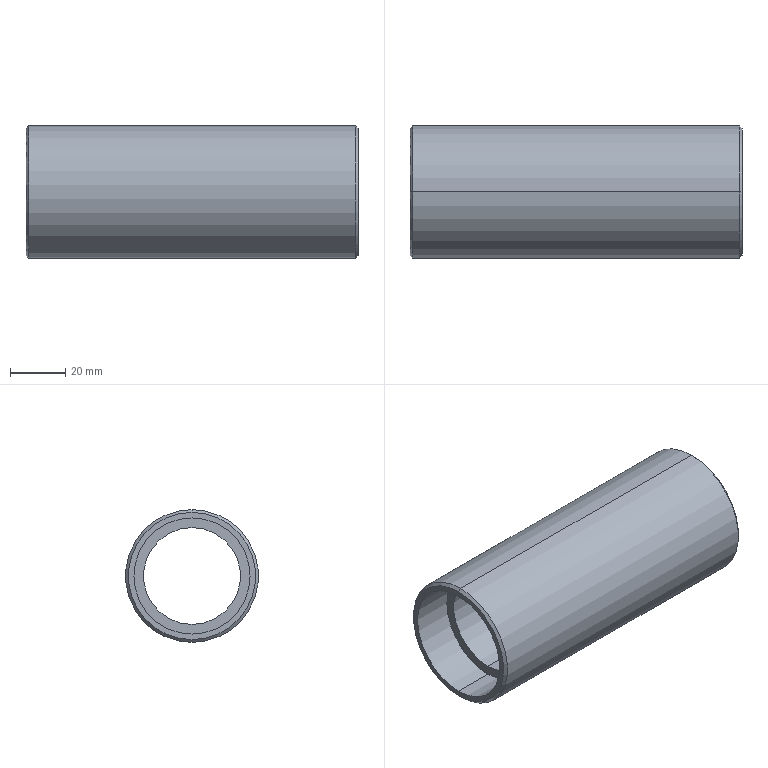Part | SolidWorks | features ICE 4, Chamfer 3, RevCut 1, Revolution 1 | 1 solid | 16 faces | box 120 x 48 x 48 mm | volume 88845 mm3 | cylinder 8 | cone 4 | plane 4 | commonest cylinder face diameters 42 x4 35 x2 48 x2
STEP:
#1=CARTESIAN_POINT('',(120.,0.,-23.));
#2=VERTEX_POINT('',#1);
#3=CARTESIAN_POINT('',(120.,0.,23.));
#4=VERTEX_POINT('',#3);
#5=CARTESIAN_POINT('',(120.,0.,0.));
#6=DIRECTION('',(1.,0.,0.));
#7=DIRECTION('',(0.,0.,-1.));
#8=AXIS2_PLACEMENT_3D('',#5,#6,#7);
#9=CIRCLE('',#8,23.);
#10=EDGE_CURVE('',#2,#4,#9,.T.);
#11=ORIENTED_EDGE('',*,*,#10,.F.);
#12=CARTESIAN_POINT('',(119.,0.,-24.));
#13=VERTEX_POINT('',#12);
#14=CARTESIAN_POINT('',(119.,0.,-24.));
#15=DIRECTION('',(-0.7071,0.,-0.7071));
#16=VECTOR('',#15,1000.);
#17=LINE('',#14,#16);
#18=EDGE_CURVE('',#2,#13,#17,.T.);
#19=ORIENTED_EDGE('',*,*,#18,.T.);
#20=CARTESIAN_POINT('',(119.,0.,24.));
#21=VERTEX_POINT('',#20);
#22=CARTESIAN_POINT('',(119.,0.,0.));
#23=DIRECTION('',(-1.,0.,0.));
#24=DIRECTION('',(0.,0.,-1.));
#25=AXIS2_PLACEMENT_3D('',#22,#23,#24);
#26=CIRCLE('',#25,24.);
#27=EDGE_CURVE('',#21,#13,#26,.T.);
#28=ORIENTED_EDGE('',*,*,#27,.F.);
#29=CARTESIAN_POINT('',(119.,0.,24.));
#30=DIRECTION('',(-0.7071,0.,0.7071));
#31=VECTOR('',#30,1000.);
#32=LINE('',#29,#31);
#33=EDGE_CURVE('',#4,#21,#32,.T.);
#34=ORIENTED_EDGE('',*,*,#33,.F.);
#35=EDGE_LOOP('',(#11,#19,#28,#34));
#36=FACE_OUTER_BOUND('',#35,.T.);
#37=CARTESIAN_POINT('',(119.,0.,0.));
#38=DIRECTION('',(-1.,0.,0.));
#39=DIRECTION('',(0.,0.,1.));
#40=AXIS2_PLACEMENT_3D('',#37,#38,#39);
#41=CONICAL_SURFACE('',#40,24.,0.7854);
#42=ADVANCED_FACE('',(#36),#41,.T.);
#43=CARTESIAN_POINT('',(0.,0.,23.));
#44=VERTEX_POINT('',#43);
#45=CARTESIAN_POINT('',(0.,0.,-23.));
#46=VERTEX_POINT('',#45);
#47=CARTESIAN_POINT('',(0.,0.,0.));
#48=DIRECTION('',(-1.,0.,0.));
#49=DIRECTION('',(0.,0.,1.));
#50=AXIS2_PLACEMENT_3D('',#47,#48,#49);
#51=CIRCLE('',#50,23.);
#52=EDGE_CURVE('',#44,#46,#51,.T.);
#53=ORIENTED_EDGE('',*,*,#52,.F.);
#54=CARTESIAN_POINT('',(1.,0.,24.));
#55=VERTEX_POINT('',#54);
#56=CARTESIAN_POINT('',(0.,0.,23.));
#57=DIRECTION('',(0.7071,0.,0.7071));
#58=VECTOR('',#57,1000.);
#59=LINE('',#56,#58);
#60=EDGE_CURVE('',#44,#55,#59,.T.);
#61=ORIENTED_EDGE('',*,*,#60,.T.);
#62=CARTESIAN_POINT('',(1.,0.,-24.));
#63=VERTEX_POINT('',#62);
#64=CARTESIAN_POINT('',(1.,0.,0.));
#65=DIRECTION('',(1.,0.,0.));
#66=DIRECTION('',(0.,0.,1.));
#67=AXIS2_PLACEMENT_3D('',#64,#65,#66);
#68=CIRCLE('',#67,24.);
#69=EDGE_CURVE('',#63,#55,#68,.T.);
#70=ORIENTED_EDGE('',*,*,#69,.F.);
#71=CARTESIAN_POINT('',(0.,0.,-23.));
#72=DIRECTION('',(0.7071,0.,-0.7071));
#73=VECTOR('',#72,1000.);
#74=LINE('',#71,#73);
#75=EDGE_CURVE('',#46,#63,#74,.T.);
#76=ORIENTED_EDGE('',*,*,#75,.F.);
#77=EDGE_LOOP('',(#53,#61,#70,#76));
#78=FACE_OUTER_BOUND('',#77,.T.);
#79=CARTESIAN_POINT('',(0.,0.,0.));
#80=DIRECTION('',(1.,0.,0.));
#81=DIRECTION('',(0.,0.,-1.));
#82=AXIS2_PLACEMENT_3D('',#79,#80,#81);
#83=CONICAL_SURFACE('',#82,23.,0.7854);
#84=ADVANCED_FACE('',(#78),#83,.T.);
#85=ORIENTED_EDGE('',*,*,#27,.T.);
#86=CARTESIAN_POINT('',(120.,0.,-24.));
#87=DIRECTION('',(-1.,0.,0.));
#88=VECTOR('',#87,1000.);
#89=LINE('',#86,#88);
#90=EDGE_CURVE('',#13,#63,#89,.T.);
#91=ORIENTED_EDGE('',*,*,#90,.T.);
#92=ORIENTED_EDGE('',*,*,#69,.T.);
#93=CARTESIAN_POINT('',(120.,0.,24.));
#94=DIRECTION('',(-1.,0.,0.));
#95=VECTOR('',#94,1000.);
#96=LINE('',#93,#95);
#97=EDGE_CURVE('',#21,#55,#96,.T.);
#98=ORIENTED_EDGE('',*,*,#97,.F.);
#99=EDGE_LOOP('',(#85,#91,#92,#98));
#100=FACE_OUTER_BOUND('',#99,.T.);
#101=CARTESIAN_POINT('',(120.,0.,0.));
#102=DIRECTION('',(-1.,0.,0.));
#103=DIRECTION('',(0.,0.,1.));
#104=AXIS2_PLACEMENT_3D('',#101,#102,#103);
#105=CYLINDRICAL_SURFACE('',#104,24.);
#106=ADVANCED_FACE('',(#100),#105,.T.);
#107=CARTESIAN_POINT('',(15.,0.,-17.5));
#108=VERTEX_POINT('',#107);
#109=CARTESIAN_POINT('',(15.,0.,17.5));
#110=VERTEX_POINT('',#109);
#111=CARTESIAN_POINT('',(15.,0.,0.));
#112=DIRECTION('',(-1.,0.,0.));
#113=DIRECTION('',(0.,0.,1.));
#114=AXIS2_PLACEMENT_3D('',#111,#112,#113);
#115=CIRCLE('',#114,17.5);
#116=EDGE_CURVE('',#108,#110,#115,.T.);
#117=ORIENTED_EDGE('',*,*,#116,.T.);
#118=CARTESIAN_POINT('',(105.,0.,17.5));
#119=VERTEX_POINT('',#118);
#120=CARTESIAN_POINT('',(0.,0.,17.5));
#121=DIRECTION('',(1.,0.,0.));
#122=VECTOR('',#121,1000.);
#123=LINE('',#120,#122);
#124=EDGE_CURVE('',#110,#119,#123,.T.);
#125=ORIENTED_EDGE('',*,*,#124,.T.);
#126=CARTESIAN_POINT('',(105.,0.,-17.5));
#127=VERTEX_POINT('',#126);
#128=CARTESIAN_POINT('',(105.,0.,0.));
#129=DIRECTION('',(1.,0.,0.));
#130=DIRECTION('',(0.,0.,-1.));
#131=AXIS2_PLACEMENT_3D('',#128,#129,#130);
#132=CIRCLE('',#131,17.5);
#133=EDGE_CURVE('',#119,#127,#132,.T.);
#134=ORIENTED_EDGE('',*,*,#133,.T.);
#135=CARTESIAN_POINT('',(0.,0.,-17.5));
#136=DIRECTION('',(1.,0.,0.));
#137=VECTOR('',#136,1000.);
#138=LINE('',#135,#137);
#139=EDGE_CURVE('',#108,#127,#138,.T.);
#140=ORIENTED_EDGE('',*,*,#139,.F.);
#141=EDGE_LOOP('',(#117,#125,#134,#140));
#142=FACE_OUTER_BOUND('',#141,.T.);
#143=CARTESIAN_POINT('',(0.,0.,0.));
#144=DIRECTION('',(1.,0.,0.));
#145=DIRECTION('',(0.,0.,-1.));
#146=AXIS2_PLACEMENT_3D('',#143,#144,#145);
#147=CYLINDRICAL_SURFACE('',#146,17.5);
#148=ADVANCED_FACE('',(#142),#147,.F.);
#149=CARTESIAN_POINT('',(105.,0.,21.));
#150=VERTEX_POINT('',#149);
#151=CARTESIAN_POINT('',(105.,0.,-21.));
#152=VERTEX_POINT('',#151);
#153=CARTESIAN_POINT('',(105.,0.,0.));
#154=DIRECTION('',(1.,0.,0.));
#155=DIRECTION('',(0.,0.,-1.));
#156=AXIS2_PLACEMENT_3D('',#153,#154,#155);
#157=CIRCLE('',#156,21.);
#158=EDGE_CURVE('',#150,#152,#157,.T.);
#159=ORIENTED_EDGE('',*,*,#158,.F.);
#160=CARTESIAN_POINT('',(120.,0.,21.));
#161=VERTEX_POINT('',#160);
#162=CARTESIAN_POINT('',(105.,0.,21.));
#163=DIRECTION('',(1.,0.,0.));
#164=VECTOR('',#163,1000.);
#165=LINE('',#162,#164);
#166=EDGE_CURVE('',#150,#161,#165,.T.);
#167=ORIENTED_EDGE('',*,*,#166,.T.);
#168=CARTESIAN_POINT('',(120.,0.,-21.));
#169=VERTEX_POINT('',#168);
#170=CARTESIAN_POINT('',(120.,0.,0.));
#171=DIRECTION('',(1.,0.,0.));
#172=DIRECTION('',(0.,0.,-1.));
#173=AXIS2_PLACEMENT_3D('',#170,#171,#172);
#174=CIRCLE('',#173,21.);
#175=EDGE_CURVE('',#161,#169,#174,.T.);
#176=ORIENTED_EDGE('',*,*,#175,.T.);
#177=CARTESIAN_POINT('',(105.,0.,-21.));
#178=DIRECTION('',(1.,0.,0.));
#179=VECTOR('',#178,1000.);
#180=LINE('',#177,#179);
#181=EDGE_CURVE('',#152,#169,#180,.T.);
#182=ORIENTED_EDGE('',*,*,#181,.F.);
#183=EDGE_LOOP('',(#159,#167,#176,#182));
#184=FACE_OUTER_BOUND('',#183,.T.);
#185=CARTESIAN_POINT('',(105.,0.,0.));
#186=DIRECTION('',(1.,0.,0.));
#187=DIRECTION('',(0.,0.,-1.));
#188=AXIS2_PLACEMENT_3D('',#185,#186,#187);
#189=CYLINDRICAL_SURFACE('',#188,21.);
#190=ADVANCED_FACE('',(#184),#189,.F.);
#191=CARTESIAN_POINT('',(15.,0.,-21.));
#192=VERTEX_POINT('',#191);
#193=CARTESIAN_POINT('',(15.,0.,21.));
#194=VERTEX_POINT('',#193);
#195=CARTESIAN_POINT('',(15.,0.,0.));
#196=DIRECTION('',(-1.,0.,0.));
#197=DIRECTION('',(0.,0.,1.));
#198=AXIS2_PLACEMENT_3D('',#195,#196,#197);
#199=CIRCLE('',#198,21.);
#200=EDGE_CURVE('',#192,#194,#199,.T.);
#201=ORIENTED_EDGE('',*,*,#200,.F.);
#202=CARTESIAN_POINT('',(0.,0.,-21.));
#203=VERTEX_POINT('',#202);
#204=CARTESIAN_POINT('',(15.,0.,-21.));
#205=DIRECTION('',(-1.,0.,0.));
#206=VECTOR('',#205,1000.);
#207=LINE('',#204,#206);
#208=EDGE_CURVE('',#192,#203,#207,.T.);
#209=ORIENTED_EDGE('',*,*,#208,.T.);
#210=CARTESIAN_POINT('',(0.,0.,21.));
#211=VERTEX_POINT('',#210);
#212=CARTESIAN_POINT('',(0.,0.,0.));
#213=DIRECTION('',(-1.,0.,0.));
#214=DIRECTION('',(0.,0.,1.));
#215=AXIS2_PLACEMENT_3D('',#212,#213,#214);
#216=CIRCLE('',#215,21.);
#217=EDGE_CURVE('',#203,#211,#216,.T.);
#218=ORIENTED_EDGE('',*,*,#217,.T.);
#219=CARTESIAN_POINT('',(15.,0.,21.));
#220=DIRECTION('',(-1.,0.,0.));
#221=VECTOR('',#220,1000.);
#222=LINE('',#219,#221);
#223=EDGE_CURVE('',#194,#211,#222,.T.);
#224=ORIENTED_EDGE('',*,*,#223,.F.);
#225=EDGE_LOOP('',(#201,#209,#218,#224));
#226=FACE_OUTER_BOUND('',#225,.T.);
#227=CARTESIAN_POINT('',(15.,0.,0.));
#228=DIRECTION('',(-1.,0.,0.));
#229=DIRECTION('',(0.,0.,1.));
#230=AXIS2_PLACEMENT_3D('',#227,#228,#229);
#231=CYLINDRICAL_SURFACE('',#230,21.);
#232=ADVANCED_FACE('',(#226),#231,.F.);
#233=CARTESIAN_POINT('',(0.,0.,0.));
#234=DIRECTION('',(-1.,0.,0.));
#235=DIRECTION('',(0.,0.,1.));
#236=AXIS2_PLACEMENT_3D('',#233,#234,#235);
#237=CIRCLE('',#236,23.);
#238=EDGE_CURVE('',#46,#44,#237,.T.);
#239=ORIENTED_EDGE('',*,*,#238,.T.);
#240=ORIENTED_EDGE('',*,*,#52,.T.);
#241=EDGE_LOOP('',(#239,#240));
#242=FACE_OUTER_BOUND('',#241,.T.);
#243=CARTESIAN_POINT('',(0.,0.,0.));
#244=DIRECTION('',(-1.,0.,0.));
#245=DIRECTION('',(0.,0.,1.));
#246=AXIS2_PLACEMENT_3D('',#243,#244,#245);
#247=CIRCLE('',#246,21.);
#248=EDGE_CURVE('',#211,#203,#247,.T.);
#249=ORIENTED_EDGE('',*,*,#248,.F.);
#250=ORIENTED_EDGE('',*,*,#217,.F.);
#251=EDGE_LOOP('',(#249,#250));
#252=FACE_BOUND('',#251,.T.);
#253=CARTESIAN_POINT('',(0.,0.,0.));
#254=DIRECTION('',(-1.,0.,0.));
#255=DIRECTION('',(0.,0.,1.));
#256=AXIS2_PLACEMENT_3D('',#253,#254,#255);
#257=PLANE('',#256);
#258=ADVANCED_FACE('',(#242,#252),#257,.T.);
#259=CARTESIAN_POINT('',(120.,0.,0.));
#260=DIRECTION('',(1.,0.,0.));
#261=DIRECTION('',(0.,0.,-1.));
#262=AXIS2_PLACEMENT_3D('',#259,#260,#261);
#263=CIRCLE('',#262,23.);
#264=EDGE_CURVE('',#4,#2,#263,.T.);
#265=ORIENTED_EDGE('',*,*,#264,.T.);
#266=ORIENTED_EDGE('',*,*,#10,.T.);
#267=EDGE_LOOP('',(#265,#266));
#268=FACE_OUTER_BOUND('',#267,.T.);
#269=CARTESIAN_POINT('',(120.,0.,0.));
#270=DIRECTION('',(1.,0.,0.));
#271=DIRECTION('',(0.,0.,-1.));
#272=AXIS2_PLACEMENT_3D('',#269,#270,#271);
#273=CIRCLE('',#272,21.);
#274=EDGE_CURVE('',#169,#161,#273,.T.);
#275=ORIENTED_EDGE('',*,*,#274,.F.);
#276=ORIENTED_EDGE('',*,*,#175,.F.);
#277=EDGE_LOOP('',(#275,#276));
#278=FACE_BOUND('',#277,.T.);
#279=CARTESIAN_POINT('',(120.,30.,0.));
#280=DIRECTION('',(1.,0.,0.));
#281=DIRECTION('',(0.,0.,-1.));
#282=AXIS2_PLACEMENT_3D('',#279,#280,#281);
#283=PLANE('',#282);
#284=ADVANCED_FACE('',(#268,#278),#283,.T.);
#285=ORIENTED_EDGE('',*,*,#208,.F.);
#286=CARTESIAN_POINT('',(15.,0.,0.));
#287=DIRECTION('',(-1.,0.,0.));
#288=DIRECTION('',(0.,0.,1.));
#289=AXIS2_PLACEMENT_3D('',#286,#287,#288);
#290=CIRCLE('',#289,21.);
#291=EDGE_CURVE('',#194,#192,#290,.T.);
#292=ORIENTED_EDGE('',*,*,#291,.F.);
#293=ORIENTED_EDGE('',*,*,#223,.T.);
#294=ORIENTED_EDGE('',*,*,#248,.T.);
#295=EDGE_LOOP('',(#285,#292,#293,#294));
#296=FACE_OUTER_BOUND('',#295,.T.);
#297=CARTESIAN_POINT('',(15.,0.,0.));
#298=DIRECTION('',(-1.,0.,0.));
#299=DIRECTION('',(0.,0.,1.));
#300=AXIS2_PLACEMENT_3D('',#297,#298,#299);
#301=CYLINDRICAL_SURFACE('',#300,21.);
#302=ADVANCED_FACE('',(#296),#301,.F.);
#303=ORIENTED_EDGE('',*,*,#116,.F.);
#304=CARTESIAN_POINT('',(15.,0.,0.));
#305=DIRECTION('',(-1.,0.,0.));
#306=DIRECTION('',(0.,0.,1.));
#307=AXIS2_PLACEMENT_3D('',#304,#305,#306);
#308=CIRCLE('',#307,17.5);
#309=EDGE_CURVE('',#110,#108,#308,.T.);
#310=ORIENTED_EDGE('',*,*,#309,.F.);
#311=EDGE_LOOP('',(#303,#310));
#312=FACE_BOUND('',#311,.T.);
#313=ORIENTED_EDGE('',*,*,#291,.T.);
#314=ORIENTED_EDGE('',*,*,#200,.T.);
#315=EDGE_LOOP('',(#313,#314));
#316=FACE_OUTER_BOUND('',#315,.T.);
#317=CARTESIAN_POINT('',(15.,0.,0.));
#318=DIRECTION('',(-1.,0.,0.));
#319=DIRECTION('',(0.,0.,1.));
#320=AXIS2_PLACEMENT_3D('',#317,#318,#319);
#321=PLANE('',#320);
#322=ADVANCED_FACE('',(#312,#316),#321,.T.);
#323=ORIENTED_EDGE('',*,*,#166,.F.);
#324=CARTESIAN_POINT('',(105.,0.,0.));
#325=DIRECTION('',(1.,0.,0.));
#326=DIRECTION('',(0.,0.,-1.));
#327=AXIS2_PLACEMENT_3D('',#324,#325,#326);
#328=CIRCLE('',#327,21.);
#329=EDGE_CURVE('',#152,#150,#328,.T.);
#330=ORIENTED_EDGE('',*,*,#329,.F.);
#331=ORIENTED_EDGE('',*,*,#181,.T.);
#332=ORIENTED_EDGE('',*,*,#274,.T.);
#333=EDGE_LOOP('',(#323,#330,#331,#332));
#334=FACE_OUTER_BOUND('',#333,.T.);
#335=CARTESIAN_POINT('',(105.,0.,0.));
#336=DIRECTION('',(1.,0.,0.));
#337=DIRECTION('',(0.,0.,-1.));
#338=AXIS2_PLACEMENT_3D('',#335,#336,#337);
#339=CYLINDRICAL_SURFACE('',#338,21.);
#340=ADVANCED_FACE('',(#334),#339,.F.);
#341=CARTESIAN_POINT('',(105.,0.,0.));
#342=DIRECTION('',(1.,0.,0.));
#343=DIRECTION('',(0.,0.,-1.));
#344=AXIS2_PLACEMENT_3D('',#341,#342,#343);
#345=CIRCLE('',#344,17.5);
#346=EDGE_CURVE('',#127,#119,#345,.T.);
#347=ORIENTED_EDGE('',*,*,#346,.F.);
#348=ORIENTED_EDGE('',*,*,#133,.F.);
#349=EDGE_LOOP('',(#347,#348));
#350=FACE_BOUND('',#349,.T.);
#351=ORIENTED_EDGE('',*,*,#329,.T.);
#352=ORIENTED_EDGE('',*,*,#158,.T.);
#353=EDGE_LOOP('',(#351,#352));
#354=FACE_OUTER_BOUND('',#353,.T.);
#355=CARTESIAN_POINT('',(105.,0.,0.));
#356=DIRECTION('',(1.,0.,0.));
#357=DIRECTION('',(0.,0.,-1.));
#358=AXIS2_PLACEMENT_3D('',#355,#356,#357);
#359=PLANE('',#358);
#360=ADVANCED_FACE('',(#350,#354),#359,.T.);
#361=ORIENTED_EDGE('',*,*,#124,.F.);
#362=ORIENTED_EDGE('',*,*,#309,.T.);
#363=ORIENTED_EDGE('',*,*,#139,.T.);
#364=ORIENTED_EDGE('',*,*,#346,.T.);
#365=EDGE_LOOP('',(#361,#362,#363,#364));
#366=FACE_OUTER_BOUND('',#365,.T.);
#367=CARTESIAN_POINT('',(0.,0.,0.));
#368=DIRECTION('',(1.,0.,0.));
#369=DIRECTION('',(0.,0.,-1.));
#370=AXIS2_PLACEMENT_3D('',#367,#368,#369);
#371=CYLINDRICAL_SURFACE('',#370,17.5);
#372=ADVANCED_FACE('',(#366),#371,.F.);
#373=ORIENTED_EDGE('',*,*,#90,.F.);
#374=CARTESIAN_POINT('',(119.,0.,0.));
#375=DIRECTION('',(-1.,0.,0.));
#376=DIRECTION('',(0.,0.,-1.));
#377=AXIS2_PLACEMENT_3D('',#374,#375,#376);
#378=CIRCLE('',#377,24.);
#379=EDGE_CURVE('',#13,#21,#378,.T.);
#380=ORIENTED_EDGE('',*,*,#379,.T.);
#381=ORIENTED_EDGE('',*,*,#97,.T.);
#382=CARTESIAN_POINT('',(1.,0.,0.));
#383=DIRECTION('',(1.,0.,0.));
#384=DIRECTION('',(0.,0.,1.));
#385=AXIS2_PLACEMENT_3D('',#382,#383,#384);
#386=CIRCLE('',#385,24.);
#387=EDGE_CURVE('',#55,#63,#386,.T.);
#388=ORIENTED_EDGE('',*,*,#387,.T.);
#389=EDGE_LOOP('',(#373,#380,#381,#388));
#390=FACE_OUTER_BOUND('',#389,.T.);
#391=CARTESIAN_POINT('',(120.,0.,0.));
#392=DIRECTION('',(-1.,0.,0.));
#393=DIRECTION('',(0.,0.,1.));
#394=AXIS2_PLACEMENT_3D('',#391,#392,#393);
#395=CYLINDRICAL_SURFACE('',#394,24.);
#396=ADVANCED_FACE('',(#390),#395,.T.);
#397=ORIENTED_EDGE('',*,*,#60,.F.);
#398=ORIENTED_EDGE('',*,*,#238,.F.);
#399=ORIENTED_EDGE('',*,*,#75,.T.);
#400=ORIENTED_EDGE('',*,*,#387,.F.);
#401=EDGE_LOOP('',(#397,#398,#399,#400));
#402=FACE_OUTER_BOUND('',#401,.T.);
#403=CARTESIAN_POINT('',(0.,0.,0.));
#404=DIRECTION('',(1.,0.,0.));
#405=DIRECTION('',(0.,0.,-1.));
#406=AXIS2_PLACEMENT_3D('',#403,#404,#405);
#407=CONICAL_SURFACE('',#406,23.,0.7854);
#408=ADVANCED_FACE('',(#402),#407,.T.);
#409=ORIENTED_EDGE('',*,*,#18,.F.);
#410=ORIENTED_EDGE('',*,*,#264,.F.);
#411=ORIENTED_EDGE('',*,*,#33,.T.);
#412=ORIENTED_EDGE('',*,*,#379,.F.);
#413=EDGE_LOOP('',(#409,#410,#411,#412));
#414=FACE_OUTER_BOUND('',#413,.T.);
#415=CARTESIAN_POINT('',(119.,0.,0.));
#416=DIRECTION('',(-1.,0.,0.));
#417=DIRECTION('',(0.,0.,1.));
#418=AXIS2_PLACEMENT_3D('',#415,#416,#417);
#419=CONICAL_SURFACE('',#418,24.,0.7854);
#420=ADVANCED_FACE('',(#414),#419,.T.);
#421=CLOSED_SHELL('',(#42,#84,#106,#148,#190,#232,#258,#284,#302,#322,#340,#360,#372,#396,#408,#420));
#422=MANIFOLD_SOLID_BREP('',#421);
#423=CARTESIAN_POINT('',(0.,0.,0.));
#424=DIRECTION('',(0.,0.,1.));
#425=DIRECTION('',(1.,0.,0.));
#426=AXIS2_PLACEMENT_3D('',#423,#424,#425);
#427=(LENGTH_UNIT()NAMED_UNIT(*)SI_UNIT(.MILLI.,.METRE.));
#428=UNCERTAINTY_MEASURE_WITH_UNIT(LENGTH_MEASURE(0.00001),#427,'','');
#429=(NAMED_UNIT(*)PLANE_ANGLE_UNIT()SI_UNIT($,.RADIAN.));
#430=(NAMED_UNIT(*)SI_UNIT($,.STERADIAN.)SOLID_ANGLE_UNIT());
#431=(GEOMETRIC_REPRESENTATION_CONTEXT(3)GLOBAL_UNCERTAINTY_ASSIGNED_CONTEXT((#428))GLOBAL_UNIT_ASSIGNED_CONTEXT((#427,#429,#430))REPRESENTATION_CONTEXT('',''));
#432=ADVANCED_BREP_SHAPE_REPRESENTATION('',(#422,#426),#431);